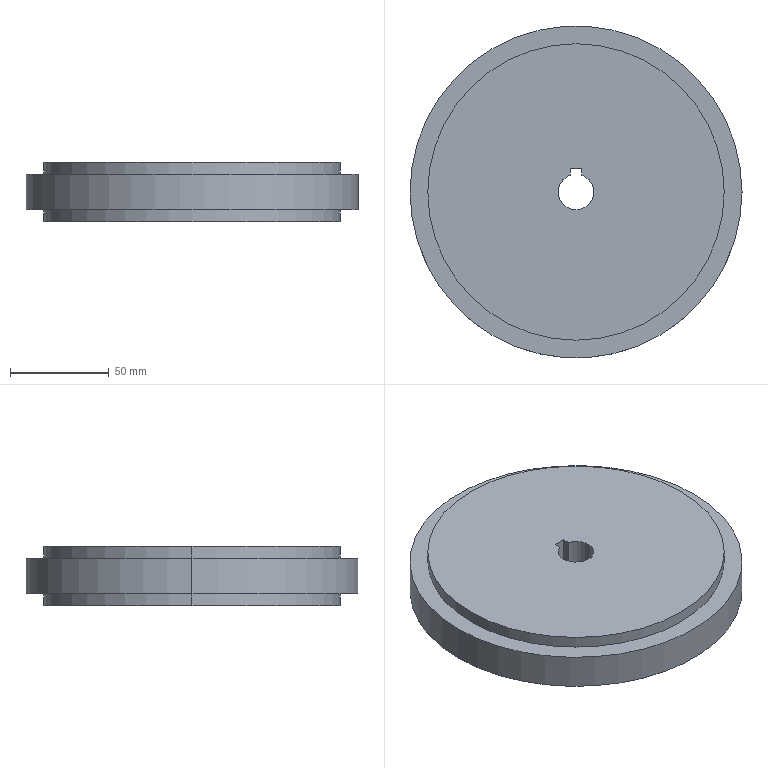Part | NX | features BREP 1 | 1 solid | 16 faces | box 168 x 168 x 30 mm | volume 602860 mm3 | cylinder 9 | plane 7 | commonest cylinder face diameters 150 x4 18 x3 168 x2
STEP:
#1=CARTESIAN_POINT('',(-9.,0.,-30.));
#2=VERTEX_POINT('',#1);
#3=CARTESIAN_POINT('',(9.,0.,-30.));
#4=VERTEX_POINT('',#3);
#5=CARTESIAN_POINT('',(0.,0.,-30.));
#6=DIRECTION('',(0.,0.,1.));
#7=DIRECTION('',(1.,0.,0.));
#8=AXIS2_PLACEMENT_3D('',#5,#6,#7);
#9=CIRCLE('',#8,9.);
#10=EDGE_CURVE('',#2,#4,#9,.T.);
#11=ORIENTED_EDGE('',*,*,#10,.F.);
#12=CARTESIAN_POINT('',(-9.,0.,0.));
#13=VERTEX_POINT('',#12);
#14=CARTESIAN_POINT('',(-9.,0.,0.));
#15=DIRECTION('',(0.,0.,1.));
#16=VECTOR('',#15,1000.);
#17=LINE('',#14,#16);
#18=EDGE_CURVE('',#2,#13,#17,.T.);
#19=ORIENTED_EDGE('',*,*,#18,.T.);
#20=CARTESIAN_POINT('',(9.,0.,0.));
#21=VERTEX_POINT('',#20);
#22=CARTESIAN_POINT('',(0.,0.,0.));
#23=DIRECTION('',(0.,0.,1.));
#24=DIRECTION('',(1.,0.,0.));
#25=AXIS2_PLACEMENT_3D('',#22,#23,#24);
#26=CIRCLE('',#25,9.);
#27=EDGE_CURVE('',#13,#21,#26,.T.);
#28=ORIENTED_EDGE('',*,*,#27,.T.);
#29=CARTESIAN_POINT('',(9.,0.,0.));
#30=DIRECTION('',(0.,0.,1.));
#31=VECTOR('',#30,1000.);
#32=LINE('',#29,#31);
#33=EDGE_CURVE('',#4,#21,#32,.T.);
#34=ORIENTED_EDGE('',*,*,#33,.F.);
#35=EDGE_LOOP('',(#11,#19,#28,#34));
#36=FACE_BOUND('',#35,.T.);
#37=CARTESIAN_POINT('',(0.,0.,0.));
#38=DIRECTION('',(0.,0.,1.));
#39=DIRECTION('',(-1.,0.,0.));
#40=AXIS2_PLACEMENT_3D('',#37,#38,#39);
#41=CYLINDRICAL_SURFACE('',#40,9.);
#42=ADVANCED_FACE('',(#36),#41,.F.);
#43=CARTESIAN_POINT('',(3.,8.485,-30.));
#44=VERTEX_POINT('',#43);
#45=CARTESIAN_POINT('',(0.,0.,-30.));
#46=DIRECTION('',(0.,0.,1.));
#47=DIRECTION('',(1.,0.,0.));
#48=AXIS2_PLACEMENT_3D('',#45,#46,#47);
#49=CIRCLE('',#48,9.);
#50=EDGE_CURVE('',#4,#44,#49,.T.);
#51=ORIENTED_EDGE('',*,*,#50,.F.);
#52=ORIENTED_EDGE('',*,*,#33,.T.);
#53=CARTESIAN_POINT('',(3.,8.485,0.));
#54=VERTEX_POINT('',#53);
#55=CARTESIAN_POINT('',(0.,0.,0.));
#56=DIRECTION('',(0.,0.,1.));
#57=DIRECTION('',(1.,0.,0.));
#58=AXIS2_PLACEMENT_3D('',#55,#56,#57);
#59=CIRCLE('',#58,9.);
#60=EDGE_CURVE('',#21,#54,#59,.T.);
#61=ORIENTED_EDGE('',*,*,#60,.T.);
#62=CARTESIAN_POINT('',(3.,8.485,-30.));
#63=DIRECTION('',(0.,0.,1.));
#64=VECTOR('',#63,1000.);
#65=LINE('',#62,#64);
#66=EDGE_CURVE('',#44,#54,#65,.T.);
#67=ORIENTED_EDGE('',*,*,#66,.F.);
#68=EDGE_LOOP('',(#51,#52,#61,#67));
#69=FACE_BOUND('',#68,.T.);
#70=CARTESIAN_POINT('',(0.,0.,0.));
#71=DIRECTION('',(0.,0.,1.));
#72=DIRECTION('',(-1.,0.,0.));
#73=AXIS2_PLACEMENT_3D('',#70,#71,#72);
#74=CYLINDRICAL_SURFACE('',#73,9.);
#75=ADVANCED_FACE('',(#69),#74,.F.);
#76=CARTESIAN_POINT('',(75.,0.,-6.));
#77=VERTEX_POINT('',#76);
#78=CARTESIAN_POINT('',(-75.,0.,-6.));
#79=VERTEX_POINT('',#78);
#80=CARTESIAN_POINT('',(0.,0.,-6.));
#81=DIRECTION('',(0.,0.,1.));
#82=DIRECTION('',(1.,0.,0.));
#83=AXIS2_PLACEMENT_3D('',#80,#81,#82);
#84=CIRCLE('',#83,75.);
#85=EDGE_CURVE('',#77,#79,#84,.T.);
#86=ORIENTED_EDGE('',*,*,#85,.T.);
#87=CARTESIAN_POINT('',(-75.,0.,0.));
#88=VERTEX_POINT('',#87);
#89=CARTESIAN_POINT('',(-75.,0.,0.));
#90=DIRECTION('',(0.,0.,1.));
#91=VECTOR('',#90,1000.);
#92=LINE('',#89,#91);
#93=EDGE_CURVE('',#79,#88,#92,.T.);
#94=ORIENTED_EDGE('',*,*,#93,.T.);
#95=CARTESIAN_POINT('',(75.,0.,0.));
#96=VERTEX_POINT('',#95);
#97=CARTESIAN_POINT('',(0.,0.,0.));
#98=DIRECTION('',(0.,0.,1.));
#99=DIRECTION('',(1.,0.,0.));
#100=AXIS2_PLACEMENT_3D('',#97,#98,#99);
#101=CIRCLE('',#100,75.);
#102=EDGE_CURVE('',#96,#88,#101,.T.);
#103=ORIENTED_EDGE('',*,*,#102,.F.);
#104=CARTESIAN_POINT('',(75.,0.,0.));
#105=DIRECTION('',(0.,0.,1.));
#106=VECTOR('',#105,1000.);
#107=LINE('',#104,#106);
#108=EDGE_CURVE('',#77,#96,#107,.T.);
#109=ORIENTED_EDGE('',*,*,#108,.F.);
#110=EDGE_LOOP('',(#86,#94,#103,#109));
#111=FACE_BOUND('',#110,.T.);
#112=CARTESIAN_POINT('',(0.,0.,0.));
#113=DIRECTION('',(0.,0.,1.));
#114=DIRECTION('',(-1.,0.,0.));
#115=AXIS2_PLACEMENT_3D('',#112,#113,#114);
#116=CYLINDRICAL_SURFACE('',#115,75.);
#117=ADVANCED_FACE('',(#111),#116,.T.);
#118=CARTESIAN_POINT('',(84.,0.,-24.));
#119=VERTEX_POINT('',#118);
#120=CARTESIAN_POINT('',(-84.,0.,-24.));
#121=VERTEX_POINT('',#120);
#122=CARTESIAN_POINT('',(0.,0.,-24.));
#123=DIRECTION('',(0.,0.,1.));
#124=DIRECTION('',(1.,0.,0.));
#125=AXIS2_PLACEMENT_3D('',#122,#123,#124);
#126=CIRCLE('',#125,84.);
#127=EDGE_CURVE('',#119,#121,#126,.T.);
#128=ORIENTED_EDGE('',*,*,#127,.T.);
#129=CARTESIAN_POINT('',(-84.,0.,-6.));
#130=VERTEX_POINT('',#129);
#131=CARTESIAN_POINT('',(-84.,0.,0.));
#132=DIRECTION('',(0.,0.,1.));
#133=VECTOR('',#132,1000.);
#134=LINE('',#131,#133);
#135=EDGE_CURVE('',#121,#130,#134,.T.);
#136=ORIENTED_EDGE('',*,*,#135,.T.);
#137=CARTESIAN_POINT('',(84.,0.,-6.));
#138=VERTEX_POINT('',#137);
#139=CARTESIAN_POINT('',(0.,0.,-6.));
#140=DIRECTION('',(0.,0.,1.));
#141=DIRECTION('',(1.,0.,0.));
#142=AXIS2_PLACEMENT_3D('',#139,#140,#141);
#143=CIRCLE('',#142,84.);
#144=EDGE_CURVE('',#138,#130,#143,.T.);
#145=ORIENTED_EDGE('',*,*,#144,.F.);
#146=CARTESIAN_POINT('',(84.,0.,0.));
#147=DIRECTION('',(0.,0.,1.));
#148=VECTOR('',#147,1000.);
#149=LINE('',#146,#148);
#150=EDGE_CURVE('',#119,#138,#149,.T.);
#151=ORIENTED_EDGE('',*,*,#150,.F.);
#152=EDGE_LOOP('',(#128,#136,#145,#151));
#153=FACE_BOUND('',#152,.T.);
#154=CARTESIAN_POINT('',(0.,0.,0.));
#155=DIRECTION('',(0.,0.,1.));
#156=DIRECTION('',(-1.,0.,0.));
#157=AXIS2_PLACEMENT_3D('',#154,#155,#156);
#158=CYLINDRICAL_SURFACE('',#157,84.);
#159=ADVANCED_FACE('',(#153),#158,.T.);
#160=CARTESIAN_POINT('',(75.,0.,-30.));
#161=VERTEX_POINT('',#160);
#162=CARTESIAN_POINT('',(-75.,0.,-30.));
#163=VERTEX_POINT('',#162);
#164=CARTESIAN_POINT('',(0.,0.,-30.));
#165=DIRECTION('',(0.,0.,1.));
#166=DIRECTION('',(1.,0.,0.));
#167=AXIS2_PLACEMENT_3D('',#164,#165,#166);
#168=CIRCLE('',#167,75.);
#169=EDGE_CURVE('',#161,#163,#168,.T.);
#170=ORIENTED_EDGE('',*,*,#169,.T.);
#171=CARTESIAN_POINT('',(-75.,0.,-24.));
#172=VERTEX_POINT('',#171);
#173=CARTESIAN_POINT('',(-75.,0.,0.));
#174=DIRECTION('',(0.,0.,1.));
#175=VECTOR('',#174,1000.);
#176=LINE('',#173,#175);
#177=EDGE_CURVE('',#163,#172,#176,.T.);
#178=ORIENTED_EDGE('',*,*,#177,.T.);
#179=CARTESIAN_POINT('',(75.,0.,-24.));
#180=VERTEX_POINT('',#179);
#181=CARTESIAN_POINT('',(0.,0.,-24.));
#182=DIRECTION('',(0.,0.,1.));
#183=DIRECTION('',(1.,0.,0.));
#184=AXIS2_PLACEMENT_3D('',#181,#182,#183);
#185=CIRCLE('',#184,75.);
#186=EDGE_CURVE('',#180,#172,#185,.T.);
#187=ORIENTED_EDGE('',*,*,#186,.F.);
#188=CARTESIAN_POINT('',(75.,0.,0.));
#189=DIRECTION('',(0.,0.,1.));
#190=VECTOR('',#189,1000.);
#191=LINE('',#188,#190);
#192=EDGE_CURVE('',#161,#180,#191,.T.);
#193=ORIENTED_EDGE('',*,*,#192,.F.);
#194=EDGE_LOOP('',(#170,#178,#187,#193));
#195=FACE_BOUND('',#194,.T.);
#196=CARTESIAN_POINT('',(0.,0.,0.));
#197=DIRECTION('',(0.,0.,1.));
#198=DIRECTION('',(-1.,0.,0.));
#199=AXIS2_PLACEMENT_3D('',#196,#197,#198);
#200=CYLINDRICAL_SURFACE('',#199,75.);
#201=ADVANCED_FACE('',(#195),#200,.T.);
#202=ORIENTED_EDGE('',*,*,#177,.F.);
#203=CARTESIAN_POINT('',(0.,0.,-30.));
#204=DIRECTION('',(0.,0.,1.));
#205=DIRECTION('',(1.,0.,0.));
#206=AXIS2_PLACEMENT_3D('',#203,#204,#205);
#207=CIRCLE('',#206,75.);
#208=EDGE_CURVE('',#163,#161,#207,.T.);
#209=ORIENTED_EDGE('',*,*,#208,.T.);
#210=ORIENTED_EDGE('',*,*,#192,.T.);
#211=CARTESIAN_POINT('',(0.,0.,-24.));
#212=DIRECTION('',(0.,0.,1.));
#213=DIRECTION('',(1.,0.,0.));
#214=AXIS2_PLACEMENT_3D('',#211,#212,#213);
#215=CIRCLE('',#214,75.);
#216=EDGE_CURVE('',#172,#180,#215,.T.);
#217=ORIENTED_EDGE('',*,*,#216,.F.);
#218=EDGE_LOOP('',(#202,#209,#210,#217));
#219=FACE_BOUND('',#218,.T.);
#220=CARTESIAN_POINT('',(0.,0.,0.));
#221=DIRECTION('',(0.,0.,1.));
#222=DIRECTION('',(-1.,0.,0.));
#223=AXIS2_PLACEMENT_3D('',#220,#221,#222);
#224=CYLINDRICAL_SURFACE('',#223,75.);
#225=ADVANCED_FACE('',(#219),#224,.T.);
#226=ORIENTED_EDGE('',*,*,#127,.F.);
#227=CARTESIAN_POINT('',(0.,0.,-24.));
#228=DIRECTION('',(0.,0.,1.));
#229=DIRECTION('',(1.,0.,0.));
#230=AXIS2_PLACEMENT_3D('',#227,#228,#229);
#231=CIRCLE('',#230,84.);
#232=EDGE_CURVE('',#121,#119,#231,.T.);
#233=ORIENTED_EDGE('',*,*,#232,.F.);
#234=EDGE_LOOP('',(#226,#233));
#235=FACE_BOUND('',#234,.T.);
#236=ORIENTED_EDGE('',*,*,#186,.T.);
#237=ORIENTED_EDGE('',*,*,#216,.T.);
#238=EDGE_LOOP('',(#236,#237));
#239=FACE_BOUND('',#238,.T.);
#240=CARTESIAN_POINT('',(0.,0.,-24.));
#241=DIRECTION('',(0.,0.,1.));
#242=DIRECTION('',(0.,1.,0.));
#243=AXIS2_PLACEMENT_3D('',#240,#241,#242);
#244=PLANE('',#243);
#245=ADVANCED_FACE('',(#235,#239),#244,.F.);
#246=ORIENTED_EDGE('',*,*,#135,.F.);
#247=ORIENTED_EDGE('',*,*,#232,.T.);
#248=ORIENTED_EDGE('',*,*,#150,.T.);
#249=CARTESIAN_POINT('',(0.,0.,-6.));
#250=DIRECTION('',(0.,0.,1.));
#251=DIRECTION('',(1.,0.,0.));
#252=AXIS2_PLACEMENT_3D('',#249,#250,#251);
#253=CIRCLE('',#252,84.);
#254=EDGE_CURVE('',#130,#138,#253,.T.);
#255=ORIENTED_EDGE('',*,*,#254,.F.);
#256=EDGE_LOOP('',(#246,#247,#248,#255));
#257=FACE_BOUND('',#256,.T.);
#258=CARTESIAN_POINT('',(0.,0.,0.));
#259=DIRECTION('',(0.,0.,1.));
#260=DIRECTION('',(-1.,0.,0.));
#261=AXIS2_PLACEMENT_3D('',#258,#259,#260);
#262=CYLINDRICAL_SURFACE('',#261,84.);
#263=ADVANCED_FACE('',(#257),#262,.T.);
#264=ORIENTED_EDGE('',*,*,#144,.T.);
#265=ORIENTED_EDGE('',*,*,#254,.T.);
#266=EDGE_LOOP('',(#264,#265));
#267=FACE_BOUND('',#266,.T.);
#268=ORIENTED_EDGE('',*,*,#85,.F.);
#269=CARTESIAN_POINT('',(0.,0.,-6.));
#270=DIRECTION('',(0.,0.,1.));
#271=DIRECTION('',(1.,0.,0.));
#272=AXIS2_PLACEMENT_3D('',#269,#270,#271);
#273=CIRCLE('',#272,75.);
#274=EDGE_CURVE('',#79,#77,#273,.T.);
#275=ORIENTED_EDGE('',*,*,#274,.F.);
#276=EDGE_LOOP('',(#268,#275));
#277=FACE_BOUND('',#276,.T.);
#278=CARTESIAN_POINT('',(0.,0.,-6.));
#279=DIRECTION('',(0.,0.,1.));
#280=DIRECTION('',(0.,1.,0.));
#281=AXIS2_PLACEMENT_3D('',#278,#279,#280);
#282=PLANE('',#281);
#283=ADVANCED_FACE('',(#267,#277),#282,.T.);
#284=ORIENTED_EDGE('',*,*,#93,.F.);
#285=ORIENTED_EDGE('',*,*,#274,.T.);
#286=ORIENTED_EDGE('',*,*,#108,.T.);
#287=CARTESIAN_POINT('',(0.,0.,0.));
#288=DIRECTION('',(0.,0.,1.));
#289=DIRECTION('',(1.,0.,0.));
#290=AXIS2_PLACEMENT_3D('',#287,#288,#289);
#291=CIRCLE('',#290,75.);
#292=EDGE_CURVE('',#88,#96,#291,.T.);
#293=ORIENTED_EDGE('',*,*,#292,.F.);
#294=EDGE_LOOP('',(#284,#285,#286,#293));
#295=FACE_BOUND('',#294,.T.);
#296=CARTESIAN_POINT('',(0.,0.,0.));
#297=DIRECTION('',(0.,0.,1.));
#298=DIRECTION('',(-1.,0.,0.));
#299=AXIS2_PLACEMENT_3D('',#296,#297,#298);
#300=CYLINDRICAL_SURFACE('',#299,75.);
#301=ADVANCED_FACE('',(#295),#300,.T.);
#302=ORIENTED_EDGE('',*,*,#102,.T.);
#303=ORIENTED_EDGE('',*,*,#292,.T.);
#304=EDGE_LOOP('',(#302,#303));
#305=FACE_BOUND('',#304,.T.);
#306=CARTESIAN_POINT('',(3.,12.,0.));
#307=VERTEX_POINT('',#306);
#308=CARTESIAN_POINT('',(3.,8.485,0.));
#309=DIRECTION('',(0.,1.,0.));
#310=VECTOR('',#309,1000.);
#311=LINE('',#308,#310);
#312=EDGE_CURVE('',#54,#307,#311,.T.);
#313=ORIENTED_EDGE('',*,*,#312,.F.);
#314=ORIENTED_EDGE('',*,*,#60,.F.);
#315=ORIENTED_EDGE('',*,*,#27,.F.);
#316=CARTESIAN_POINT('',(-3.,8.485,0.));
#317=VERTEX_POINT('',#316);
#318=CARTESIAN_POINT('',(0.,0.,0.));
#319=DIRECTION('',(0.,0.,1.));
#320=DIRECTION('',(1.,0.,0.));
#321=AXIS2_PLACEMENT_3D('',#318,#319,#320);
#322=CIRCLE('',#321,9.);
#323=EDGE_CURVE('',#317,#13,#322,.T.);
#324=ORIENTED_EDGE('',*,*,#323,.F.);
#325=CARTESIAN_POINT('',(-3.,12.,0.));
#326=VERTEX_POINT('',#325);
#327=CARTESIAN_POINT('',(-3.,8.485,0.));
#328=DIRECTION('',(0.,-1.,0.));
#329=VECTOR('',#328,1000.);
#330=LINE('',#327,#329);
#331=EDGE_CURVE('',#326,#317,#330,.T.);
#332=ORIENTED_EDGE('',*,*,#331,.F.);
#333=CARTESIAN_POINT('',(-3.,12.,0.));
#334=DIRECTION('',(-1.,0.,0.));
#335=VECTOR('',#334,1000.);
#336=LINE('',#333,#335);
#337=EDGE_CURVE('',#307,#326,#336,.T.);
#338=ORIENTED_EDGE('',*,*,#337,.F.);
#339=EDGE_LOOP('',(#313,#314,#315,#324,#332,#338));
#340=FACE_BOUND('',#339,.T.);
#341=CARTESIAN_POINT('',(0.,0.,0.));
#342=DIRECTION('',(0.,0.,1.));
#343=DIRECTION('',(0.,1.,0.));
#344=AXIS2_PLACEMENT_3D('',#341,#342,#343);
#345=PLANE('',#344);
#346=ADVANCED_FACE('',(#305,#340),#345,.T.);
#347=ORIENTED_EDGE('',*,*,#18,.F.);
#348=CARTESIAN_POINT('',(-3.,8.485,-30.));
#349=VERTEX_POINT('',#348);
#350=CARTESIAN_POINT('',(0.,0.,-30.));
#351=DIRECTION('',(0.,0.,1.));
#352=DIRECTION('',(1.,0.,0.));
#353=AXIS2_PLACEMENT_3D('',#350,#351,#352);
#354=CIRCLE('',#353,9.);
#355=EDGE_CURVE('',#349,#2,#354,.T.);
#356=ORIENTED_EDGE('',*,*,#355,.F.);
#357=CARTESIAN_POINT('',(-3.,8.485,-30.));
#358=DIRECTION('',(0.,0.,1.));
#359=VECTOR('',#358,1000.);
#360=LINE('',#357,#359);
#361=EDGE_CURVE('',#349,#317,#360,.T.);
#362=ORIENTED_EDGE('',*,*,#361,.T.);
#363=ORIENTED_EDGE('',*,*,#323,.T.);
#364=EDGE_LOOP('',(#347,#356,#362,#363));
#365=FACE_BOUND('',#364,.T.);
#366=CARTESIAN_POINT('',(0.,0.,0.));
#367=DIRECTION('',(0.,0.,1.));
#368=DIRECTION('',(-1.,0.,0.));
#369=AXIS2_PLACEMENT_3D('',#366,#367,#368);
#370=CYLINDRICAL_SURFACE('',#369,9.);
#371=ADVANCED_FACE('',(#365),#370,.F.);
#372=ORIENTED_EDGE('',*,*,#169,.F.);
#373=ORIENTED_EDGE('',*,*,#208,.F.);
#374=EDGE_LOOP('',(#372,#373));
#375=FACE_BOUND('',#374,.T.);
#376=ORIENTED_EDGE('',*,*,#355,.T.);
#377=ORIENTED_EDGE('',*,*,#10,.T.);
#378=ORIENTED_EDGE('',*,*,#50,.T.);
#379=CARTESIAN_POINT('',(3.,12.,-30.));
#380=VERTEX_POINT('',#379);
#381=CARTESIAN_POINT('',(3.,8.485,-30.));
#382=DIRECTION('',(0.,1.,0.));
#383=VECTOR('',#382,1000.);
#384=LINE('',#381,#383);
#385=EDGE_CURVE('',#44,#380,#384,.T.);
#386=ORIENTED_EDGE('',*,*,#385,.T.);
#387=CARTESIAN_POINT('',(-3.,12.,-30.));
#388=VERTEX_POINT('',#387);
#389=CARTESIAN_POINT('',(-3.,12.,-30.));
#390=DIRECTION('',(-1.,0.,0.));
#391=VECTOR('',#390,1000.);
#392=LINE('',#389,#391);
#393=EDGE_CURVE('',#380,#388,#392,.T.);
#394=ORIENTED_EDGE('',*,*,#393,.T.);
#395=CARTESIAN_POINT('',(-3.,8.485,-30.));
#396=DIRECTION('',(0.,-1.,0.));
#397=VECTOR('',#396,1000.);
#398=LINE('',#395,#397);
#399=EDGE_CURVE('',#388,#349,#398,.T.);
#400=ORIENTED_EDGE('',*,*,#399,.T.);
#401=EDGE_LOOP('',(#376,#377,#378,#386,#394,#400));
#402=FACE_BOUND('',#401,.T.);
#403=CARTESIAN_POINT('',(0.,0.,-30.));
#404=DIRECTION('',(0.,0.,1.));
#405=DIRECTION('',(0.,1.,0.));
#406=AXIS2_PLACEMENT_3D('',#403,#404,#405);
#407=PLANE('',#406);
#408=ADVANCED_FACE('',(#375,#402),#407,.F.);
#409=ORIENTED_EDGE('',*,*,#337,.T.);
#410=CARTESIAN_POINT('',(-3.,12.,-30.));
#411=DIRECTION('',(0.,0.,1.));
#412=VECTOR('',#411,1000.);
#413=LINE('',#410,#412);
#414=EDGE_CURVE('',#388,#326,#413,.T.);
#415=ORIENTED_EDGE('',*,*,#414,.F.);
#416=ORIENTED_EDGE('',*,*,#393,.F.);
#417=CARTESIAN_POINT('',(3.,12.,-30.));
#418=DIRECTION('',(0.,0.,1.));
#419=VECTOR('',#418,1000.);
#420=LINE('',#417,#419);
#421=EDGE_CURVE('',#380,#307,#420,.T.);
#422=ORIENTED_EDGE('',*,*,#421,.T.);
#423=EDGE_LOOP('',(#409,#415,#416,#422));
#424=FACE_BOUND('',#423,.T.);
#425=CARTESIAN_POINT('',(-3.,12.,-30.));
#426=DIRECTION('',(0.,1.,0.));
#427=DIRECTION('',(-1.,0.,0.));
#428=AXIS2_PLACEMENT_3D('',#425,#426,#427);
#429=PLANE('',#428);
#430=ADVANCED_FACE('',(#424),#429,.F.);
#431=ORIENTED_EDGE('',*,*,#312,.T.);
#432=ORIENTED_EDGE('',*,*,#421,.F.);
#433=ORIENTED_EDGE('',*,*,#385,.F.);
#434=ORIENTED_EDGE('',*,*,#66,.T.);
#435=EDGE_LOOP('',(#431,#432,#433,#434));
#436=FACE_BOUND('',#435,.T.);
#437=CARTESIAN_POINT('',(3.,8.485,-30.));
#438=DIRECTION('',(1.,0.,0.));
#439=DIRECTION('',(0.,1.,0.));
#440=AXIS2_PLACEMENT_3D('',#437,#438,#439);
#441=PLANE('',#440);
#442=ADVANCED_FACE('',(#436),#441,.F.);
#443=ORIENTED_EDGE('',*,*,#331,.T.);
#444=ORIENTED_EDGE('',*,*,#361,.F.);
#445=ORIENTED_EDGE('',*,*,#399,.F.);
#446=ORIENTED_EDGE('',*,*,#414,.T.);
#447=EDGE_LOOP('',(#443,#444,#445,#446));
#448=FACE_BOUND('',#447,.T.);
#449=CARTESIAN_POINT('',(-3.,8.485,-30.));
#450=DIRECTION('',(-1.,0.,0.));
#451=DIRECTION('',(0.,0.,-1.));
#452=AXIS2_PLACEMENT_3D('',#449,#450,#451);
#453=PLANE('',#452);
#454=ADVANCED_FACE('',(#448),#453,.F.);
#455=CLOSED_SHELL('',(#42,#75,#117,#159,#201,#225,#245,#263,#283,#301,#346,#371,#408,#430,#442,#454));
#456=MANIFOLD_SOLID_BREP('',#455);
#457=(LENGTH_UNIT()NAMED_UNIT(*)SI_UNIT(.MILLI.,.METRE.));
#458=UNCERTAINTY_MEASURE_WITH_UNIT(LENGTH_MEASURE(0.00001),#457,'','');
#459=(NAMED_UNIT(*)PLANE_ANGLE_UNIT()SI_UNIT($,.RADIAN.));
#460=(NAMED_UNIT(*)SI_UNIT($,.STERADIAN.)SOLID_ANGLE_UNIT());
#461=(GEOMETRIC_REPRESENTATION_CONTEXT(3)GLOBAL_UNCERTAINTY_ASSIGNED_CONTEXT((#458))GLOBAL_UNIT_ASSIGNED_CONTEXT((#457,#459,#460))REPRESENTATION_CONTEXT('',''));
#462=ADVANCED_BREP_SHAPE_REPRESENTATION('',(#456),#461);